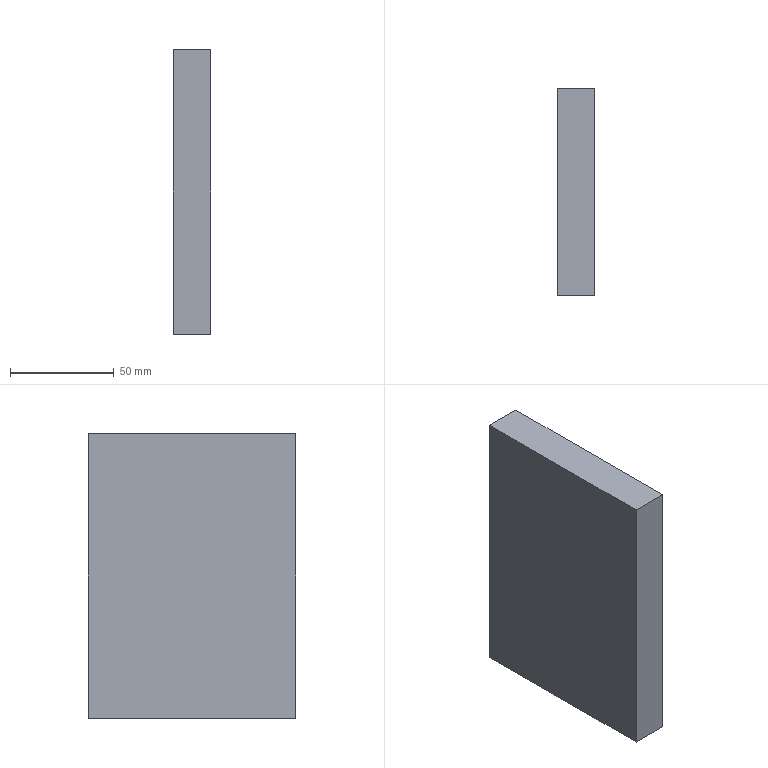Part | STEP file | Middle_part | 1 solid | 6 faces | box 18 x 100 x 137 mm | volume 246600 mm3 | plane 6
STEP:
#1=CARTESIAN_POINT('',(0.,0.,0.));
#2=DIRECTION('',(0.,0.,1.));
#3=DIRECTION('',(1.,0.,0.));
#4=AXIS2_PLACEMENT_3D('',#1,#2,#3);
#5=CARTESIAN_POINT('',(0.,-50.,68.5));
#6=VERTEX_POINT('',#5);
#7=CARTESIAN_POINT('',(18.,-50.,68.5));
#8=VERTEX_POINT('',#7);
#9=CARTESIAN_POINT('',(0.,-50.,68.5));
#10=DIRECTION('',(1.,0.,0.));
#11=VECTOR('',#10,1.);
#12=LINE('',#9,#11);
#13=CARTESIAN_POINT('',(0.,-50.,68.5));
#14=DIRECTION('',(0.,1.,0.));
#15=DIRECTION('',(0.,0.,-1.));
#16=AXIS2_PLACEMENT_3D('',#13,#14,#15);
#17=PLANE('',#16);
#18=CARTESIAN_POINT('',(0.,0.));
#19=DIRECTION('',(0.,-1.));
#20=VECTOR('',#19,1.);
#21=LINE('',#18,#20);
#22=(GEOMETRIC_REPRESENTATION_CONTEXT(2)PARAMETRIC_REPRESENTATION_CONTEXT()REPRESENTATION_CONTEXT('',''));
#23=DEFINITIONAL_REPRESENTATION('',(#21),#22);
#24=PCURVE('',#17,#23);
#25=CARTESIAN_POINT('',(0.,50.,68.5));
#26=DIRECTION('',(0.,0.,-1.));
#27=DIRECTION('',(0.,-1.,0.));
#28=AXIS2_PLACEMENT_3D('',#25,#26,#27);
#29=PLANE('',#28);
#30=CARTESIAN_POINT('',(100.,0.));
#31=DIRECTION('',(0.,-1.));
#32=VECTOR('',#31,1.);
#33=LINE('',#30,#32);
#34=(GEOMETRIC_REPRESENTATION_CONTEXT(2)PARAMETRIC_REPRESENTATION_CONTEXT()REPRESENTATION_CONTEXT('',''));
#35=DEFINITIONAL_REPRESENTATION('',(#33),#34);
#36=PCURVE('',#29,#35);
#37=SURFACE_CURVE('',#12,(#24,#36),.PCURVE_S1.);
#38=EDGE_CURVE('',#6,#8,#37,.T.);
#39=ORIENTED_EDGE('',*,*,#38,.T.);
#40=CARTESIAN_POINT('',(18.,-50.,-68.5));
#41=VERTEX_POINT('',#40);
#42=CARTESIAN_POINT('',(18.,-50.,68.5));
#43=DIRECTION('',(0.,0.,-1.));
#44=VECTOR('',#43,1.);
#45=LINE('',#42,#44);
#46=CARTESIAN_POINT('',(0.,-18.));
#47=DIRECTION('',(1.,0.));
#48=VECTOR('',#47,1.);
#49=LINE('',#46,#48);
#50=(GEOMETRIC_REPRESENTATION_CONTEXT(2)PARAMETRIC_REPRESENTATION_CONTEXT()REPRESENTATION_CONTEXT('',''));
#51=DEFINITIONAL_REPRESENTATION('',(#49),#50);
#52=PCURVE('',#17,#51);
#53=CARTESIAN_POINT('',(18.,0.,0.));
#54=DIRECTION('',(1.,0.,0.));
#55=DIRECTION('',(0.,0.,1.));
#56=AXIS2_PLACEMENT_3D('',#53,#54,#55);
#57=PLANE('',#56);
#58=CARTESIAN_POINT('',(68.5,50.));
#59=DIRECTION('',(-1.,0.));
#60=VECTOR('',#59,1.);
#61=LINE('',#58,#60);
#62=(GEOMETRIC_REPRESENTATION_CONTEXT(2)PARAMETRIC_REPRESENTATION_CONTEXT()REPRESENTATION_CONTEXT('',''));
#63=DEFINITIONAL_REPRESENTATION('',(#61),#62);
#64=PCURVE('',#57,#63);
#65=SURFACE_CURVE('',#45,(#52,#64),.PCURVE_S1.);
#66=EDGE_CURVE('',#8,#41,#65,.T.);
#67=ORIENTED_EDGE('',*,*,#66,.T.);
#68=CARTESIAN_POINT('',(0.,-50.,-68.5));
#69=VERTEX_POINT('',#68);
#70=CARTESIAN_POINT('',(0.,-50.,-68.5));
#71=DIRECTION('',(1.,0.,0.));
#72=VECTOR('',#71,1.);
#73=LINE('',#70,#72);
#74=CARTESIAN_POINT('',(137.,0.));
#75=DIRECTION('',(0.,-1.));
#76=VECTOR('',#75,1.);
#77=LINE('',#74,#76);
#78=(GEOMETRIC_REPRESENTATION_CONTEXT(2)PARAMETRIC_REPRESENTATION_CONTEXT()REPRESENTATION_CONTEXT('',''));
#79=DEFINITIONAL_REPRESENTATION('',(#77),#78);
#80=PCURVE('',#17,#79);
#81=CARTESIAN_POINT('',(0.,-50.,-68.5));
#82=DIRECTION('',(0.,0.,1.));
#83=DIRECTION('',(0.,1.,0.));
#84=AXIS2_PLACEMENT_3D('',#81,#82,#83);
#85=PLANE('',#84);
#86=CARTESIAN_POINT('',(0.,0.));
#87=DIRECTION('',(0.,-1.));
#88=VECTOR('',#87,1.);
#89=LINE('',#86,#88);
#90=(GEOMETRIC_REPRESENTATION_CONTEXT(2)PARAMETRIC_REPRESENTATION_CONTEXT()REPRESENTATION_CONTEXT('',''));
#91=DEFINITIONAL_REPRESENTATION('',(#89),#90);
#92=PCURVE('',#85,#91);
#93=SURFACE_CURVE('',#73,(#80,#92),.PCURVE_S1.);
#94=EDGE_CURVE('',#69,#41,#93,.T.);
#95=ORIENTED_EDGE('',*,*,#94,.F.);
#96=CARTESIAN_POINT('',(0.,-50.,68.5));
#97=DIRECTION('',(0.,0.,-1.));
#98=VECTOR('',#97,1.);
#99=LINE('',#96,#98);
#100=CARTESIAN_POINT('',(0.,0.));
#101=DIRECTION('',(1.,0.));
#102=VECTOR('',#101,1.);
#103=LINE('',#100,#102);
#104=(GEOMETRIC_REPRESENTATION_CONTEXT(2)PARAMETRIC_REPRESENTATION_CONTEXT()REPRESENTATION_CONTEXT('',''));
#105=DEFINITIONAL_REPRESENTATION('',(#103),#104);
#106=PCURVE('',#17,#105);
#107=CARTESIAN_POINT('',(0.,0.,0.));
#108=DIRECTION('',(1.,0.,0.));
#109=DIRECTION('',(0.,0.,1.));
#110=AXIS2_PLACEMENT_3D('',#107,#108,#109);
#111=PLANE('',#110);
#112=CARTESIAN_POINT('',(68.5,50.));
#113=DIRECTION('',(-1.,0.));
#114=VECTOR('',#113,1.);
#115=LINE('',#112,#114);
#116=(GEOMETRIC_REPRESENTATION_CONTEXT(2)PARAMETRIC_REPRESENTATION_CONTEXT()REPRESENTATION_CONTEXT('',''));
#117=DEFINITIONAL_REPRESENTATION('',(#115),#116);
#118=PCURVE('',#111,#117);
#119=SURFACE_CURVE('',#99,(#106,#118),.PCURVE_S1.);
#120=EDGE_CURVE('',#6,#69,#119,.T.);
#121=ORIENTED_EDGE('',*,*,#120,.F.);
#122=EDGE_LOOP('',(#39,#67,#95,#121));
#123=FACE_BOUND('',#122,.F.);
#124=ADVANCED_FACE('',(#123),#17,.F.);
#125=ORIENTED_EDGE('',*,*,#94,.T.);
#126=CARTESIAN_POINT('',(18.,50.,-68.5));
#127=VERTEX_POINT('',#126);
#128=CARTESIAN_POINT('',(18.,-50.,-68.5));
#129=DIRECTION('',(0.,1.,0.));
#130=VECTOR('',#129,1.);
#131=LINE('',#128,#130);
#132=CARTESIAN_POINT('',(0.,-18.));
#133=DIRECTION('',(1.,0.));
#134=VECTOR('',#133,1.);
#135=LINE('',#132,#134);
#136=(GEOMETRIC_REPRESENTATION_CONTEXT(2)PARAMETRIC_REPRESENTATION_CONTEXT()REPRESENTATION_CONTEXT('',''));
#137=DEFINITIONAL_REPRESENTATION('',(#135),#136);
#138=PCURVE('',#85,#137);
#139=CARTESIAN_POINT('',(-68.5,50.));
#140=DIRECTION('',(0.,-1.));
#141=VECTOR('',#140,1.);
#142=LINE('',#139,#141);
#143=(GEOMETRIC_REPRESENTATION_CONTEXT(2)PARAMETRIC_REPRESENTATION_CONTEXT()REPRESENTATION_CONTEXT('',''));
#144=DEFINITIONAL_REPRESENTATION('',(#142),#143);
#145=PCURVE('',#57,#144);
#146=SURFACE_CURVE('',#131,(#138,#145),.PCURVE_S1.);
#147=EDGE_CURVE('',#41,#127,#146,.T.);
#148=ORIENTED_EDGE('',*,*,#147,.T.);
#149=CARTESIAN_POINT('',(0.,50.,-68.5));
#150=VERTEX_POINT('',#149);
#151=CARTESIAN_POINT('',(0.,50.,-68.5));
#152=DIRECTION('',(1.,0.,0.));
#153=VECTOR('',#152,1.);
#154=LINE('',#151,#153);
#155=CARTESIAN_POINT('',(100.,0.));
#156=DIRECTION('',(0.,-1.));
#157=VECTOR('',#156,1.);
#158=LINE('',#155,#157);
#159=(GEOMETRIC_REPRESENTATION_CONTEXT(2)PARAMETRIC_REPRESENTATION_CONTEXT()REPRESENTATION_CONTEXT('',''));
#160=DEFINITIONAL_REPRESENTATION('',(#158),#159);
#161=PCURVE('',#85,#160);
#162=CARTESIAN_POINT('',(0.,50.,-68.5));
#163=DIRECTION('',(0.,-1.,0.));
#164=DIRECTION('',(0.,0.,1.));
#165=AXIS2_PLACEMENT_3D('',#162,#163,#164);
#166=PLANE('',#165);
#167=CARTESIAN_POINT('',(0.,0.));
#168=DIRECTION('',(0.,-1.));
#169=VECTOR('',#168,1.);
#170=LINE('',#167,#169);
#171=(GEOMETRIC_REPRESENTATION_CONTEXT(2)PARAMETRIC_REPRESENTATION_CONTEXT()REPRESENTATION_CONTEXT('',''));
#172=DEFINITIONAL_REPRESENTATION('',(#170),#171);
#173=PCURVE('',#166,#172);
#174=SURFACE_CURVE('',#154,(#161,#173),.PCURVE_S1.);
#175=EDGE_CURVE('',#150,#127,#174,.T.);
#176=ORIENTED_EDGE('',*,*,#175,.F.);
#177=CARTESIAN_POINT('',(0.,-50.,-68.5));
#178=DIRECTION('',(0.,1.,0.));
#179=VECTOR('',#178,1.);
#180=LINE('',#177,#179);
#181=CARTESIAN_POINT('',(0.,0.));
#182=DIRECTION('',(1.,0.));
#183=VECTOR('',#182,1.);
#184=LINE('',#181,#183);
#185=(GEOMETRIC_REPRESENTATION_CONTEXT(2)PARAMETRIC_REPRESENTATION_CONTEXT()REPRESENTATION_CONTEXT('',''));
#186=DEFINITIONAL_REPRESENTATION('',(#184),#185);
#187=PCURVE('',#85,#186);
#188=CARTESIAN_POINT('',(-68.5,50.));
#189=DIRECTION('',(0.,-1.));
#190=VECTOR('',#189,1.);
#191=LINE('',#188,#190);
#192=(GEOMETRIC_REPRESENTATION_CONTEXT(2)PARAMETRIC_REPRESENTATION_CONTEXT()REPRESENTATION_CONTEXT('',''));
#193=DEFINITIONAL_REPRESENTATION('',(#191),#192);
#194=PCURVE('',#111,#193);
#195=SURFACE_CURVE('',#180,(#187,#194),.PCURVE_S1.);
#196=EDGE_CURVE('',#69,#150,#195,.T.);
#197=ORIENTED_EDGE('',*,*,#196,.F.);
#198=EDGE_LOOP('',(#125,#148,#176,#197));
#199=FACE_BOUND('',#198,.F.);
#200=ADVANCED_FACE('',(#199),#85,.F.);
#201=ORIENTED_EDGE('',*,*,#175,.T.);
#202=CARTESIAN_POINT('',(18.,50.,68.5));
#203=VERTEX_POINT('',#202);
#204=CARTESIAN_POINT('',(18.,50.,-68.5));
#205=DIRECTION('',(0.,0.,1.));
#206=VECTOR('',#205,1.);
#207=LINE('',#204,#206);
#208=CARTESIAN_POINT('',(0.,-18.));
#209=DIRECTION('',(1.,0.));
#210=VECTOR('',#209,1.);
#211=LINE('',#208,#210);
#212=(GEOMETRIC_REPRESENTATION_CONTEXT(2)PARAMETRIC_REPRESENTATION_CONTEXT()REPRESENTATION_CONTEXT('',''));
#213=DEFINITIONAL_REPRESENTATION('',(#211),#212);
#214=PCURVE('',#166,#213);
#215=CARTESIAN_POINT('',(-68.5,-50.));
#216=DIRECTION('',(1.,0.));
#217=VECTOR('',#216,1.);
#218=LINE('',#215,#217);
#219=(GEOMETRIC_REPRESENTATION_CONTEXT(2)PARAMETRIC_REPRESENTATION_CONTEXT()REPRESENTATION_CONTEXT('',''));
#220=DEFINITIONAL_REPRESENTATION('',(#218),#219);
#221=PCURVE('',#57,#220);
#222=SURFACE_CURVE('',#207,(#214,#221),.PCURVE_S1.);
#223=EDGE_CURVE('',#127,#203,#222,.T.);
#224=ORIENTED_EDGE('',*,*,#223,.T.);
#225=CARTESIAN_POINT('',(0.,50.,68.5));
#226=VERTEX_POINT('',#225);
#227=CARTESIAN_POINT('',(0.,50.,68.5));
#228=DIRECTION('',(1.,0.,0.));
#229=VECTOR('',#228,1.);
#230=LINE('',#227,#229);
#231=CARTESIAN_POINT('',(137.,0.));
#232=DIRECTION('',(0.,-1.));
#233=VECTOR('',#232,1.);
#234=LINE('',#231,#233);
#235=(GEOMETRIC_REPRESENTATION_CONTEXT(2)PARAMETRIC_REPRESENTATION_CONTEXT()REPRESENTATION_CONTEXT('',''));
#236=DEFINITIONAL_REPRESENTATION('',(#234),#235);
#237=PCURVE('',#166,#236);
#238=CARTESIAN_POINT('',(0.,0.));
#239=DIRECTION('',(0.,-1.));
#240=VECTOR('',#239,1.);
#241=LINE('',#238,#240);
#242=(GEOMETRIC_REPRESENTATION_CONTEXT(2)PARAMETRIC_REPRESENTATION_CONTEXT()REPRESENTATION_CONTEXT('',''));
#243=DEFINITIONAL_REPRESENTATION('',(#241),#242);
#244=PCURVE('',#29,#243);
#245=SURFACE_CURVE('',#230,(#237,#244),.PCURVE_S1.);
#246=EDGE_CURVE('',#226,#203,#245,.T.);
#247=ORIENTED_EDGE('',*,*,#246,.F.);
#248=CARTESIAN_POINT('',(0.,50.,-68.5));
#249=DIRECTION('',(0.,0.,1.));
#250=VECTOR('',#249,1.);
#251=LINE('',#248,#250);
#252=CARTESIAN_POINT('',(0.,0.));
#253=DIRECTION('',(1.,0.));
#254=VECTOR('',#253,1.);
#255=LINE('',#252,#254);
#256=(GEOMETRIC_REPRESENTATION_CONTEXT(2)PARAMETRIC_REPRESENTATION_CONTEXT()REPRESENTATION_CONTEXT('',''));
#257=DEFINITIONAL_REPRESENTATION('',(#255),#256);
#258=PCURVE('',#166,#257);
#259=CARTESIAN_POINT('',(-68.5,-50.));
#260=DIRECTION('',(1.,0.));
#261=VECTOR('',#260,1.);
#262=LINE('',#259,#261);
#263=(GEOMETRIC_REPRESENTATION_CONTEXT(2)PARAMETRIC_REPRESENTATION_CONTEXT()REPRESENTATION_CONTEXT('',''));
#264=DEFINITIONAL_REPRESENTATION('',(#262),#263);
#265=PCURVE('',#111,#264);
#266=SURFACE_CURVE('',#251,(#258,#265),.PCURVE_S1.);
#267=EDGE_CURVE('',#150,#226,#266,.T.);
#268=ORIENTED_EDGE('',*,*,#267,.F.);
#269=EDGE_LOOP('',(#201,#224,#247,#268));
#270=FACE_BOUND('',#269,.F.);
#271=ADVANCED_FACE('',(#270),#166,.F.);
#272=ORIENTED_EDGE('',*,*,#246,.T.);
#273=CARTESIAN_POINT('',(18.,50.,68.5));
#274=DIRECTION('',(0.,-1.,0.));
#275=VECTOR('',#274,1.);
#276=LINE('',#273,#275);
#277=CARTESIAN_POINT('',(0.,-18.));
#278=DIRECTION('',(1.,0.));
#279=VECTOR('',#278,1.);
#280=LINE('',#277,#279);
#281=(GEOMETRIC_REPRESENTATION_CONTEXT(2)PARAMETRIC_REPRESENTATION_CONTEXT()REPRESENTATION_CONTEXT('',''));
#282=DEFINITIONAL_REPRESENTATION('',(#280),#281);
#283=PCURVE('',#29,#282);
#284=CARTESIAN_POINT('',(68.5,-50.));
#285=DIRECTION('',(0.,1.));
#286=VECTOR('',#285,1.);
#287=LINE('',#284,#286);
#288=(GEOMETRIC_REPRESENTATION_CONTEXT(2)PARAMETRIC_REPRESENTATION_CONTEXT()REPRESENTATION_CONTEXT('',''));
#289=DEFINITIONAL_REPRESENTATION('',(#287),#288);
#290=PCURVE('',#57,#289);
#291=SURFACE_CURVE('',#276,(#283,#290),.PCURVE_S1.);
#292=EDGE_CURVE('',#203,#8,#291,.T.);
#293=ORIENTED_EDGE('',*,*,#292,.T.);
#294=ORIENTED_EDGE('',*,*,#38,.F.);
#295=CARTESIAN_POINT('',(0.,50.,68.5));
#296=DIRECTION('',(0.,-1.,0.));
#297=VECTOR('',#296,1.);
#298=LINE('',#295,#297);
#299=CARTESIAN_POINT('',(0.,0.));
#300=DIRECTION('',(1.,0.));
#301=VECTOR('',#300,1.);
#302=LINE('',#299,#301);
#303=(GEOMETRIC_REPRESENTATION_CONTEXT(2)PARAMETRIC_REPRESENTATION_CONTEXT()REPRESENTATION_CONTEXT('',''));
#304=DEFINITIONAL_REPRESENTATION('',(#302),#303);
#305=PCURVE('',#29,#304);
#306=CARTESIAN_POINT('',(68.5,-50.));
#307=DIRECTION('',(0.,1.));
#308=VECTOR('',#307,1.);
#309=LINE('',#306,#308);
#310=(GEOMETRIC_REPRESENTATION_CONTEXT(2)PARAMETRIC_REPRESENTATION_CONTEXT()REPRESENTATION_CONTEXT('',''));
#311=DEFINITIONAL_REPRESENTATION('',(#309),#310);
#312=PCURVE('',#111,#311);
#313=SURFACE_CURVE('',#298,(#305,#312),.PCURVE_S1.);
#314=EDGE_CURVE('',#226,#6,#313,.T.);
#315=ORIENTED_EDGE('',*,*,#314,.F.);
#316=EDGE_LOOP('',(#272,#293,#294,#315));
#317=FACE_BOUND('',#316,.F.);
#318=ADVANCED_FACE('',(#317),#29,.F.);
#319=ORIENTED_EDGE('',*,*,#120,.T.);
#320=ORIENTED_EDGE('',*,*,#196,.T.);
#321=ORIENTED_EDGE('',*,*,#267,.T.);
#322=ORIENTED_EDGE('',*,*,#314,.T.);
#323=EDGE_LOOP('',(#319,#320,#321,#322));
#324=FACE_BOUND('',#323,.F.);
#325=ADVANCED_FACE('',(#324),#111,.F.);
#326=ORIENTED_EDGE('',*,*,#66,.T.);
#327=ORIENTED_EDGE('',*,*,#147,.T.);
#328=ORIENTED_EDGE('',*,*,#223,.T.);
#329=ORIENTED_EDGE('',*,*,#292,.T.);
#330=EDGE_LOOP('',(#326,#327,#328,#329));
#331=FACE_BOUND('',#330,.T.);
#332=ADVANCED_FACE('',(#331),#57,.T.);
#333=CLOSED_SHELL('',(#124,#200,#271,#318,#325,#332));
#334=MANIFOLD_SOLID_BREP('',#333);
#335=(LENGTH_UNIT()NAMED_UNIT(*)SI_UNIT(.MILLI.,.METRE.));
#336=UNCERTAINTY_MEASURE_WITH_UNIT(LENGTH_MEASURE(0.0000001),#335,'','');
#337=(NAMED_UNIT(*)PLANE_ANGLE_UNIT()SI_UNIT($,.RADIAN.));
#338=(NAMED_UNIT(*)SI_UNIT($,.STERADIAN.)SOLID_ANGLE_UNIT());
#339=(GEOMETRIC_REPRESENTATION_CONTEXT(3)GLOBAL_UNCERTAINTY_ASSIGNED_CONTEXT((#336))GLOBAL_UNIT_ASSIGNED_CONTEXT((#335,#337,#338))REPRESENTATION_CONTEXT('',''));
#340=ADVANCED_BREP_SHAPE_REPRESENTATION('',(#4,#334),#339);